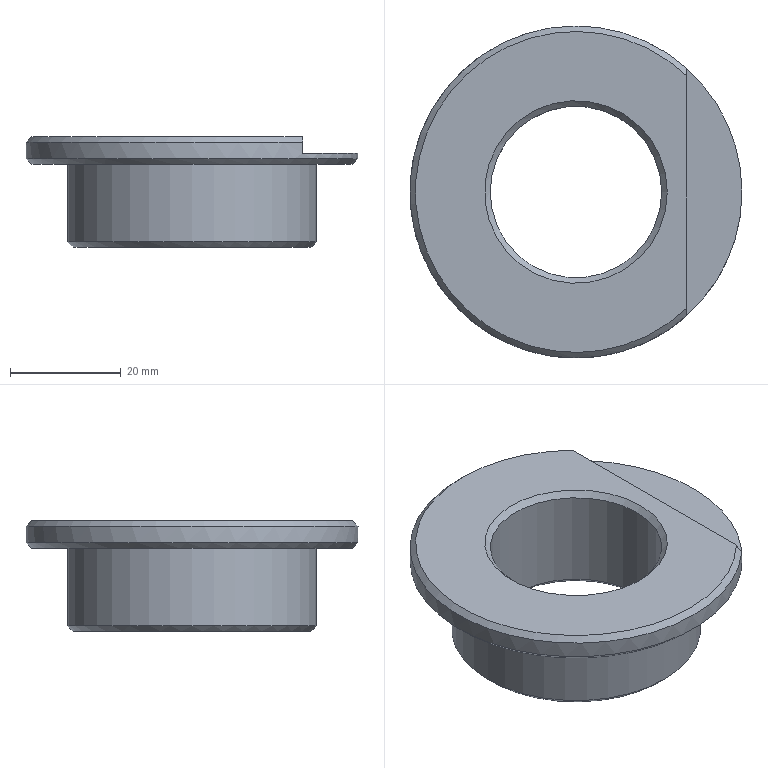Part | NX | features DATUM_CSYS 5, EXTRUDE 4, SKETCH 4, CHAMFER 1 | 1 solid | 13 faces | box 60 x 60 x 20 mm | volume 21638 mm3 | plane 5 | cone 5 | cylinder 3 | commonest cylinder face diameters 31 x1 45 x1 60 x1
STEP:
#1=CARTESIAN_POINT('',(22.5,0.,1.));
#2=VERTEX_POINT('',#1);
#3=CARTESIAN_POINT('',(0.,0.,1.));
#4=DIRECTION('',(0.,0.,1.));
#5=DIRECTION('',(1.,0.,0.));
#6=AXIS2_PLACEMENT_3D('',#3,#4,#5);
#7=CIRCLE('',#6,22.5);
#8=EDGE_CURVE('',#2,#2,#7,.T.);
#9=ORIENTED_EDGE('',*,*,#8,.T.);
#10=EDGE_LOOP('',(#9));
#11=FACE_BOUND('',#10,.T.);
#12=CARTESIAN_POINT('',(22.5,0.,15.));
#13=VERTEX_POINT('',#12);
#14=CARTESIAN_POINT('',(0.,0.,15.));
#15=DIRECTION('',(0.,0.,1.));
#16=DIRECTION('',(1.,0.,0.));
#17=AXIS2_PLACEMENT_3D('',#14,#15,#16);
#18=CIRCLE('',#17,22.5);
#19=EDGE_CURVE('',#13,#13,#18,.T.);
#20=ORIENTED_EDGE('',*,*,#19,.F.);
#21=EDGE_LOOP('',(#20));
#22=FACE_BOUND('',#21,.T.);
#23=CARTESIAN_POINT('',(0.,0.,15.));
#24=DIRECTION('',(0.,0.,-1.));
#25=DIRECTION('',(-1.,0.,0.));
#26=AXIS2_PLACEMENT_3D('',#23,#24,#25);
#27=CYLINDRICAL_SURFACE('',#26,22.5);
#28=ADVANCED_FACE('',(#11,#22),#27,.T.);
#29=CARTESIAN_POINT('',(16.5,0.,0.));
#30=VERTEX_POINT('',#29);
#31=CARTESIAN_POINT('',(0.,0.,0.));
#32=DIRECTION('',(0.,0.,1.));
#33=DIRECTION('',(1.,0.,0.));
#34=AXIS2_PLACEMENT_3D('',#31,#32,#33);
#35=CIRCLE('',#34,16.5);
#36=EDGE_CURVE('',#30,#30,#35,.T.);
#37=ORIENTED_EDGE('',*,*,#36,.T.);
#38=EDGE_LOOP('',(#37));
#39=FACE_BOUND('',#38,.T.);
#40=CARTESIAN_POINT('',(21.5,0.,0.));
#41=VERTEX_POINT('',#40);
#42=CARTESIAN_POINT('',(0.,0.,0.));
#43=DIRECTION('',(0.,0.,1.));
#44=DIRECTION('',(1.,0.,0.));
#45=AXIS2_PLACEMENT_3D('',#42,#43,#44);
#46=CIRCLE('',#45,21.5);
#47=EDGE_CURVE('',#41,#41,#46,.F.);
#48=ORIENTED_EDGE('',*,*,#47,.T.);
#49=EDGE_LOOP('',(#48));
#50=FACE_BOUND('',#49,.T.);
#51=CARTESIAN_POINT('',(0.,0.,0.));
#52=DIRECTION('',(0.,0.,1.));
#53=DIRECTION('',(1.,0.,0.));
#54=AXIS2_PLACEMENT_3D('',#51,#52,#53);
#55=PLANE('',#54);
#56=ADVANCED_FACE('',(#39,#50),#55,.F.);
#57=CARTESIAN_POINT('',(20.,-22.361,19.));
#58=VERTEX_POINT('',#57);
#59=CARTESIAN_POINT('',(20.,22.361,19.));
#60=VERTEX_POINT('',#59);
#61=CARTESIAN_POINT('',(0.,0.,19.));
#62=DIRECTION('',(0.,0.,1.));
#63=DIRECTION('',(1.,0.,0.));
#64=AXIS2_PLACEMENT_3D('',#61,#62,#63);
#65=CIRCLE('',#64,30.);
#66=EDGE_CURVE('',#58,#60,#65,.F.);
#67=ORIENTED_EDGE('',*,*,#66,.T.);
#68=CARTESIAN_POINT('',(20.,22.361,17.));
#69=VERTEX_POINT('',#68);
#70=CARTESIAN_POINT('',(20.,22.361,20.));
#71=DIRECTION('',(0.,0.,-1.));
#72=VECTOR('',#71,1000.);
#73=LINE('',#70,#72);
#74=EDGE_CURVE('',#60,#69,#73,.T.);
#75=ORIENTED_EDGE('',*,*,#74,.T.);
#76=CARTESIAN_POINT('',(20.,-22.361,17.));
#77=VERTEX_POINT('',#76);
#78=CARTESIAN_POINT('',(0.,0.,17.));
#79=DIRECTION('',(0.,0.,1.));
#80=DIRECTION('',(1.,0.,0.));
#81=AXIS2_PLACEMENT_3D('',#78,#79,#80);
#82=CIRCLE('',#81,30.);
#83=EDGE_CURVE('',#77,#69,#82,.T.);
#84=ORIENTED_EDGE('',*,*,#83,.F.);
#85=CARTESIAN_POINT('',(20.,-22.361,20.));
#86=DIRECTION('',(0.,0.,-1.));
#87=VECTOR('',#86,1000.);
#88=LINE('',#85,#87);
#89=EDGE_CURVE('',#77,#58,#88,.F.);
#90=ORIENTED_EDGE('',*,*,#89,.T.);
#91=EDGE_LOOP('',(#67,#75,#84,#90));
#92=FACE_BOUND('',#91,.T.);
#93=CARTESIAN_POINT('',(30.,0.,16.));
#94=VERTEX_POINT('',#93);
#95=CARTESIAN_POINT('',(0.,0.,16.));
#96=DIRECTION('',(0.,0.,1.));
#97=DIRECTION('',(1.,0.,0.));
#98=AXIS2_PLACEMENT_3D('',#95,#96,#97);
#99=CIRCLE('',#98,30.);
#100=EDGE_CURVE('',#94,#94,#99,.T.);
#101=ORIENTED_EDGE('',*,*,#100,.T.);
#102=EDGE_LOOP('',(#101));
#103=FACE_BOUND('',#102,.T.);
#104=CARTESIAN_POINT('',(0.,0.,20.));
#105=DIRECTION('',(0.,0.,-1.));
#106=DIRECTION('',(-1.,0.,0.));
#107=AXIS2_PLACEMENT_3D('',#104,#105,#106);
#108=CYLINDRICAL_SURFACE('',#107,30.);
#109=ADVANCED_FACE('',(#92,#103),#108,.T.);
#110=CARTESIAN_POINT('',(20.,21.,20.));
#111=VERTEX_POINT('',#110);
#112=CARTESIAN_POINT('',(20.,-21.,20.));
#113=VERTEX_POINT('',#112);
#114=CARTESIAN_POINT('',(20.,30.,20.));
#115=DIRECTION('',(0.,-1.,0.));
#116=VECTOR('',#115,1000.);
#117=LINE('',#114,#116);
#118=EDGE_CURVE('',#111,#113,#117,.T.);
#119=ORIENTED_EDGE('',*,*,#118,.F.);
#120=CARTESIAN_POINT('',(0.,0.,20.));
#121=DIRECTION('',(0.,0.,1.));
#122=DIRECTION('',(1.,0.,0.));
#123=AXIS2_PLACEMENT_3D('',#120,#121,#122);
#124=CIRCLE('',#123,29.);
#125=EDGE_CURVE('',#111,#113,#124,.T.);
#126=ORIENTED_EDGE('',*,*,#125,.T.);
#127=EDGE_LOOP('',(#119,#126));
#128=FACE_BOUND('',#127,.T.);
#129=CARTESIAN_POINT('',(16.5,0.,20.));
#130=VERTEX_POINT('',#129);
#131=CARTESIAN_POINT('',(0.,0.,20.));
#132=DIRECTION('',(0.,0.,1.));
#133=DIRECTION('',(1.,0.,0.));
#134=AXIS2_PLACEMENT_3D('',#131,#132,#133);
#135=CIRCLE('',#134,16.5);
#136=EDGE_CURVE('',#130,#130,#135,.F.);
#137=ORIENTED_EDGE('',*,*,#136,.T.);
#138=EDGE_LOOP('',(#137));
#139=FACE_BOUND('',#138,.T.);
#140=CARTESIAN_POINT('',(0.,0.,20.));
#141=DIRECTION('',(0.,0.,1.));
#142=DIRECTION('',(1.,0.,0.));
#143=AXIS2_PLACEMENT_3D('',#140,#141,#142);
#144=PLANE('',#143);
#145=ADVANCED_FACE('',(#128,#139),#144,.T.);
#146=CARTESIAN_POINT('',(29.,0.,15.));
#147=VERTEX_POINT('',#146);
#148=CARTESIAN_POINT('',(0.,0.,15.));
#149=DIRECTION('',(0.,0.,1.));
#150=DIRECTION('',(1.,0.,0.));
#151=AXIS2_PLACEMENT_3D('',#148,#149,#150);
#152=CIRCLE('',#151,29.);
#153=EDGE_CURVE('',#147,#147,#152,.F.);
#154=ORIENTED_EDGE('',*,*,#153,.T.);
#155=EDGE_LOOP('',(#154));
#156=FACE_BOUND('',#155,.T.);
#157=ORIENTED_EDGE('',*,*,#19,.T.);
#158=EDGE_LOOP('',(#157));
#159=FACE_BOUND('',#158,.T.);
#160=CARTESIAN_POINT('',(0.,0.,15.));
#161=DIRECTION('',(0.,0.,1.));
#162=DIRECTION('',(1.,0.,0.));
#163=AXIS2_PLACEMENT_3D('',#160,#161,#162);
#164=PLANE('',#163);
#165=ADVANCED_FACE('',(#156,#159),#164,.F.);
#166=CARTESIAN_POINT('',(15.5,0.,19.));
#167=VERTEX_POINT('',#166);
#168=CARTESIAN_POINT('',(0.,0.,19.));
#169=DIRECTION('',(0.,0.,1.));
#170=DIRECTION('',(1.,0.,0.));
#171=AXIS2_PLACEMENT_3D('',#168,#169,#170);
#172=CIRCLE('',#171,15.5);
#173=EDGE_CURVE('',#167,#167,#172,.T.);
#174=ORIENTED_EDGE('',*,*,#173,.T.);
#175=EDGE_LOOP('',(#174));
#176=FACE_BOUND('',#175,.T.);
#177=CARTESIAN_POINT('',(15.5,0.,1.));
#178=VERTEX_POINT('',#177);
#179=CARTESIAN_POINT('',(0.,0.,1.));
#180=DIRECTION('',(0.,0.,1.));
#181=DIRECTION('',(1.,0.,0.));
#182=AXIS2_PLACEMENT_3D('',#179,#180,#181);
#183=CIRCLE('',#182,15.5);
#184=EDGE_CURVE('',#178,#178,#183,.F.);
#185=ORIENTED_EDGE('',*,*,#184,.T.);
#186=EDGE_LOOP('',(#185));
#187=FACE_BOUND('',#186,.T.);
#188=CARTESIAN_POINT('',(0.,0.,-30.));
#189=DIRECTION('',(0.,0.,1.));
#190=DIRECTION('',(1.,0.,0.));
#191=AXIS2_PLACEMENT_3D('',#188,#189,#190);
#192=CYLINDRICAL_SURFACE('',#191,15.5);
#193=ADVANCED_FACE('',(#176,#187),#192,.F.);
#194=ORIENTED_EDGE('',*,*,#136,.F.);
#195=EDGE_LOOP('',(#194));
#196=FACE_BOUND('',#195,.T.);
#197=ORIENTED_EDGE('',*,*,#173,.F.);
#198=EDGE_LOOP('',(#197));
#199=FACE_BOUND('',#198,.T.);
#200=CARTESIAN_POINT('',(0.,0.,19.));
#201=DIRECTION('',(0.,0.,1.));
#202=DIRECTION('',(1.,0.,0.));
#203=AXIS2_PLACEMENT_3D('',#200,#201,#202);
#204=CONICAL_SURFACE('',#203,15.5,0.7854);
#205=ADVANCED_FACE('',(#196,#199),#204,.F.);
#206=ORIENTED_EDGE('',*,*,#184,.F.);
#207=EDGE_LOOP('',(#206));
#208=FACE_BOUND('',#207,.T.);
#209=ORIENTED_EDGE('',*,*,#36,.F.);
#210=EDGE_LOOP('',(#209));
#211=FACE_BOUND('',#210,.T.);
#212=CARTESIAN_POINT('',(0.,0.,0.));
#213=DIRECTION('',(0.,0.,-1.));
#214=DIRECTION('',(-1.,0.,0.));
#215=AXIS2_PLACEMENT_3D('',#212,#213,#214);
#216=CONICAL_SURFACE('',#215,16.5,0.7854);
#217=ADVANCED_FACE('',(#208,#211),#216,.F.);
#218=ORIENTED_EDGE('',*,*,#47,.F.);
#219=EDGE_LOOP('',(#218));
#220=FACE_BOUND('',#219,.T.);
#221=ORIENTED_EDGE('',*,*,#8,.F.);
#222=EDGE_LOOP('',(#221));
#223=FACE_BOUND('',#222,.T.);
#224=CARTESIAN_POINT('',(0.,0.,1.));
#225=DIRECTION('',(0.,0.,1.));
#226=DIRECTION('',(1.,0.,0.));
#227=AXIS2_PLACEMENT_3D('',#224,#225,#226);
#228=CONICAL_SURFACE('',#227,22.5,0.7854);
#229=ADVANCED_FACE('',(#220,#223),#228,.T.);
#230=ORIENTED_EDGE('',*,*,#153,.F.);
#231=EDGE_LOOP('',(#230));
#232=FACE_BOUND('',#231,.T.);
#233=ORIENTED_EDGE('',*,*,#100,.F.);
#234=EDGE_LOOP('',(#233));
#235=FACE_BOUND('',#234,.T.);
#236=CARTESIAN_POINT('',(0.,0.,16.));
#237=DIRECTION('',(0.,0.,1.));
#238=DIRECTION('',(1.,0.,0.));
#239=AXIS2_PLACEMENT_3D('',#236,#237,#238);
#240=CONICAL_SURFACE('',#239,30.,0.7854);
#241=ADVANCED_FACE('',(#232,#235),#240,.T.);
#242=CARTESIAN_POINT('',(20.,22.361,19.));
#243=CARTESIAN_POINT('',(20.,21.909,19.336));
#244=CARTESIAN_POINT('',(20.,21.456,19.67));
#245=CARTESIAN_POINT('',(20.,21.,20.));
#246=B_SPLINE_CURVE_WITH_KNOTS('',3,(#242,#243,#244,#245),.UNSPECIFIED.,.F.,.F.,(4,4),(0.05426,0.05595),.UNSPECIFIED.);
#247=EDGE_CURVE('',#60,#111,#246,.T.);
#248=ORIENTED_EDGE('',*,*,#247,.F.);
#249=ORIENTED_EDGE('',*,*,#66,.F.);
#250=CARTESIAN_POINT('',(20.,-21.,20.));
#251=CARTESIAN_POINT('',(20.,-21.456,19.67));
#252=CARTESIAN_POINT('',(20.,-21.909,19.337));
#253=CARTESIAN_POINT('',(20.,-22.361,19.));
#254=B_SPLINE_CURVE_WITH_KNOTS('',3,(#250,#251,#252,#253),.UNSPECIFIED.,.F.,.F.,(4,4),(0.1024,0.1041),.UNSPECIFIED.);
#255=EDGE_CURVE('',#113,#58,#254,.T.);
#256=ORIENTED_EDGE('',*,*,#255,.F.);
#257=ORIENTED_EDGE('',*,*,#125,.F.);
#258=EDGE_LOOP('',(#248,#249,#256,#257));
#259=FACE_BOUND('',#258,.T.);
#260=CARTESIAN_POINT('',(0.,0.,20.));
#261=DIRECTION('',(0.,0.,-1.));
#262=DIRECTION('',(-1.,0.,0.));
#263=AXIS2_PLACEMENT_3D('',#260,#261,#262);
#264=CONICAL_SURFACE('',#263,29.,0.7854);
#265=ADVANCED_FACE('',(#259),#264,.T.);
#266=ORIENTED_EDGE('',*,*,#83,.T.);
#267=CARTESIAN_POINT('',(20.,30.,17.));
#268=DIRECTION('',(0.,-1.,0.));
#269=VECTOR('',#268,1000.);
#270=LINE('',#267,#269);
#271=EDGE_CURVE('',#77,#69,#270,.F.);
#272=ORIENTED_EDGE('',*,*,#271,.F.);
#273=EDGE_LOOP('',(#266,#272));
#274=FACE_BOUND('',#273,.T.);
#275=CARTESIAN_POINT('',(0.,0.,17.));
#276=DIRECTION('',(0.,0.,1.));
#277=DIRECTION('',(1.,0.,0.));
#278=AXIS2_PLACEMENT_3D('',#275,#276,#277);
#279=PLANE('',#278);
#280=ADVANCED_FACE('',(#274),#279,.T.);
#281=ORIENTED_EDGE('',*,*,#247,.T.);
#282=ORIENTED_EDGE('',*,*,#118,.T.);
#283=ORIENTED_EDGE('',*,*,#255,.T.);
#284=ORIENTED_EDGE('',*,*,#89,.F.);
#285=ORIENTED_EDGE('',*,*,#271,.T.);
#286=ORIENTED_EDGE('',*,*,#74,.F.);
#287=EDGE_LOOP('',(#281,#282,#283,#284,#285,#286));
#288=FACE_BOUND('',#287,.T.);
#289=CARTESIAN_POINT('',(20.,30.,17.));
#290=DIRECTION('',(-1.,0.,0.));
#291=DIRECTION('',(0.,0.,1.));
#292=AXIS2_PLACEMENT_3D('',#289,#290,#291);
#293=PLANE('',#292);
#294=ADVANCED_FACE('',(#288),#293,.F.);
#295=CLOSED_SHELL('',(#28,#56,#109,#145,#165,#193,#205,#217,#229,#241,#265,#280,#294));
#296=MANIFOLD_SOLID_BREP('',#295);
#297=(LENGTH_UNIT()NAMED_UNIT(*)SI_UNIT(.MILLI.,.METRE.));
#298=UNCERTAINTY_MEASURE_WITH_UNIT(LENGTH_MEASURE(0.0508),#297,'','');
#299=(NAMED_UNIT(*)PLANE_ANGLE_UNIT()SI_UNIT($,.RADIAN.));
#300=(NAMED_UNIT(*)SI_UNIT($,.STERADIAN.)SOLID_ANGLE_UNIT());
#301=(GEOMETRIC_REPRESENTATION_CONTEXT(3)GLOBAL_UNCERTAINTY_ASSIGNED_CONTEXT((#298))GLOBAL_UNIT_ASSIGNED_CONTEXT((#297,#299,#300))REPRESENTATION_CONTEXT('',''));
#302=ADVANCED_BREP_SHAPE_REPRESENTATION('',(#296),#301);